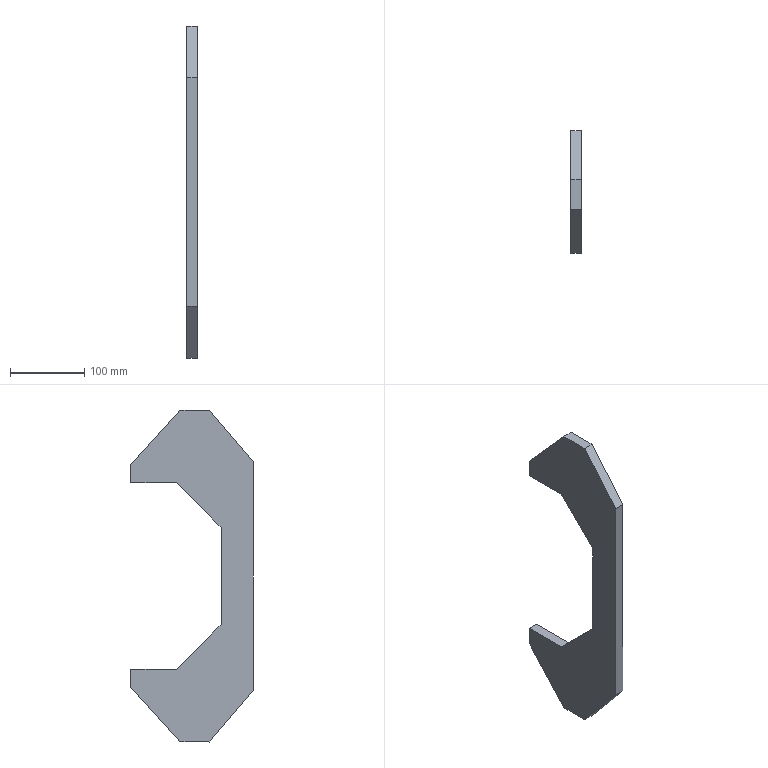Part | NX | features REPLACE_FACE 4, DATUM_CSYS 3, EXTRUDE 2, LINKED_FACE 2, SKETCH 2, BREP 1 | 1 solid | 16 faces | box 14 x 165.316 x 448 mm | volume 531264 mm3 | plane 16
STEP:
#1=CARTESIAN_POINT('',(116.,-146.,154.));
#2=VERTEX_POINT('',#1);
#3=CARTESIAN_POINT('',(116.,-146.,-154.));
#4=VERTEX_POINT('',#3);
#5=CARTESIAN_POINT('',(116.,-146.,154.));
#6=DIRECTION('',(0.,0.,-1.));
#7=VECTOR('',#6,1000.);
#8=LINE('',#5,#7);
#9=EDGE_CURVE('',#2,#4,#8,.T.);
#10=ORIENTED_EDGE('',*,*,#9,.F.);
#11=CARTESIAN_POINT('',(102.,-146.,154.));
#12=VERTEX_POINT('',#11);
#13=CARTESIAN_POINT('',(102.,-146.,154.));
#14=DIRECTION('',(1.,0.,0.));
#15=VECTOR('',#14,1000.);
#16=LINE('',#13,#15);
#17=EDGE_CURVE('',#12,#2,#16,.T.);
#18=ORIENTED_EDGE('',*,*,#17,.F.);
#19=CARTESIAN_POINT('',(102.,-146.,-154.));
#20=VERTEX_POINT('',#19);
#21=CARTESIAN_POINT('',(102.,-146.,154.));
#22=DIRECTION('',(0.,0.,-1.));
#23=VECTOR('',#22,1000.);
#24=LINE('',#21,#23);
#25=EDGE_CURVE('',#12,#20,#24,.T.);
#26=ORIENTED_EDGE('',*,*,#25,.T.);
#27=CARTESIAN_POINT('',(102.,-146.,-154.));
#28=DIRECTION('',(1.,0.,0.));
#29=VECTOR('',#28,1000.);
#30=LINE('',#27,#29);
#31=EDGE_CURVE('',#20,#4,#30,.T.);
#32=ORIENTED_EDGE('',*,*,#31,.T.);
#33=EDGE_LOOP('',(#10,#18,#26,#32));
#34=FACE_BOUND('',#33,.T.);
#35=CARTESIAN_POINT('',(102.,-146.,154.));
#36=DIRECTION('',(0.,-1.,0.));
#37=DIRECTION('',(0.,0.,-1.));
#38=AXIS2_PLACEMENT_3D('',#35,#36,#37);
#39=PLANE('',#38);
#40=ADVANCED_FACE('',(#34),#39,.T.);
#41=CARTESIAN_POINT('',(116.,-87.,-224.));
#42=VERTEX_POINT('',#41);
#43=CARTESIAN_POINT('',(116.,-146.,-154.));
#44=DIRECTION('',(0.,0.6445,-0.7646));
#45=VECTOR('',#44,1000.);
#46=LINE('',#43,#45);
#47=EDGE_CURVE('',#4,#42,#46,.T.);
#48=ORIENTED_EDGE('',*,*,#47,.F.);
#49=ORIENTED_EDGE('',*,*,#31,.F.);
#50=CARTESIAN_POINT('',(102.,-87.,-224.));
#51=VERTEX_POINT('',#50);
#52=CARTESIAN_POINT('',(102.,-146.,-154.));
#53=DIRECTION('',(0.,0.6445,-0.7646));
#54=VECTOR('',#53,1000.);
#55=LINE('',#52,#54);
#56=EDGE_CURVE('',#20,#51,#55,.T.);
#57=ORIENTED_EDGE('',*,*,#56,.T.);
#58=CARTESIAN_POINT('',(102.,-87.,-224.));
#59=DIRECTION('',(1.,0.,0.));
#60=VECTOR('',#59,1000.);
#61=LINE('',#58,#60);
#62=EDGE_CURVE('',#51,#42,#61,.T.);
#63=ORIENTED_EDGE('',*,*,#62,.T.);
#64=EDGE_LOOP('',(#48,#49,#57,#63));
#65=FACE_BOUND('',#64,.T.);
#66=CARTESIAN_POINT('',(102.,-146.,-154.));
#67=DIRECTION('',(0.,-0.7646,-0.6445));
#68=DIRECTION('',(0.,0.6445,-0.7646));
#69=AXIS2_PLACEMENT_3D('',#66,#67,#68);
#70=PLANE('',#69);
#71=ADVANCED_FACE('',(#65),#70,.T.);
#72=CARTESIAN_POINT('',(116.,-47.,-224.));
#73=VERTEX_POINT('',#72);
#74=CARTESIAN_POINT('',(116.,-87.,-224.));
#75=DIRECTION('',(0.,1.,0.));
#76=VECTOR('',#75,1000.);
#77=LINE('',#74,#76);
#78=EDGE_CURVE('',#42,#73,#77,.T.);
#79=ORIENTED_EDGE('',*,*,#78,.F.);
#80=ORIENTED_EDGE('',*,*,#62,.F.);
#81=CARTESIAN_POINT('',(102.,-47.,-224.));
#82=VERTEX_POINT('',#81);
#83=CARTESIAN_POINT('',(102.,-87.,-224.));
#84=DIRECTION('',(0.,1.,0.));
#85=VECTOR('',#84,1000.);
#86=LINE('',#83,#85);
#87=EDGE_CURVE('',#51,#82,#86,.T.);
#88=ORIENTED_EDGE('',*,*,#87,.T.);
#89=CARTESIAN_POINT('',(102.,-47.,-224.));
#90=DIRECTION('',(1.,0.,0.));
#91=VECTOR('',#90,1000.);
#92=LINE('',#89,#91);
#93=EDGE_CURVE('',#82,#73,#92,.T.);
#94=ORIENTED_EDGE('',*,*,#93,.T.);
#95=EDGE_LOOP('',(#79,#80,#88,#94));
#96=FACE_BOUND('',#95,.T.);
#97=CARTESIAN_POINT('',(102.,-87.,-224.));
#98=DIRECTION('',(0.,0.,-1.));
#99=DIRECTION('',(-1.,0.,0.));
#100=AXIS2_PLACEMENT_3D('',#97,#98,#99);
#101=PLANE('',#100);
#102=ADVANCED_FACE('',(#96),#101,.T.);
#103=CARTESIAN_POINT('',(116.,19.316,-150.316));
#104=VERTEX_POINT('',#103);
#105=CARTESIAN_POINT('',(116.,-47.,-224.));
#106=DIRECTION('',(0.,0.669,0.7433));
#107=VECTOR('',#106,1000.);
#108=LINE('',#105,#107);
#109=EDGE_CURVE('',#73,#104,#108,.T.);
#110=ORIENTED_EDGE('',*,*,#109,.F.);
#111=ORIENTED_EDGE('',*,*,#93,.F.);
#112=CARTESIAN_POINT('',(102.,19.316,-150.316));
#113=VERTEX_POINT('',#112);
#114=CARTESIAN_POINT('',(102.,-47.,-224.));
#115=DIRECTION('',(0.,0.669,0.7433));
#116=VECTOR('',#115,1000.);
#117=LINE('',#114,#116);
#118=EDGE_CURVE('',#82,#113,#117,.T.);
#119=ORIENTED_EDGE('',*,*,#118,.T.);
#120=CARTESIAN_POINT('',(102.,19.316,-150.316));
#121=DIRECTION('',(1.,0.,0.));
#122=VECTOR('',#121,1000.);
#123=LINE('',#120,#122);
#124=EDGE_CURVE('',#104,#113,#123,.F.);
#125=ORIENTED_EDGE('',*,*,#124,.F.);
#126=EDGE_LOOP('',(#110,#111,#119,#125));
#127=FACE_BOUND('',#126,.T.);
#128=CARTESIAN_POINT('',(102.,-47.,-224.));
#129=DIRECTION('',(0.,0.7433,-0.669));
#130=DIRECTION('',(0.,0.669,0.7433));
#131=AXIS2_PLACEMENT_3D('',#128,#129,#130);
#132=PLANE('',#131);
#133=ADVANCED_FACE('',(#127),#132,.T.);
#134=CARTESIAN_POINT('',(116.,19.316,-126.));
#135=VERTEX_POINT('',#134);
#136=CARTESIAN_POINT('',(116.,-42.5,-126.));
#137=VERTEX_POINT('',#136);
#138=CARTESIAN_POINT('',(116.,16.,-126.));
#139=DIRECTION('',(0.,-1.,0.));
#140=VECTOR('',#139,1000.);
#141=LINE('',#138,#140);
#142=EDGE_CURVE('',#135,#137,#141,.T.);
#143=ORIENTED_EDGE('',*,*,#142,.F.);
#144=CARTESIAN_POINT('',(102.,19.316,-126.));
#145=VERTEX_POINT('',#144);
#146=CARTESIAN_POINT('',(116.,19.316,-126.));
#147=DIRECTION('',(-1.,0.,0.));
#148=VECTOR('',#147,1000.);
#149=LINE('',#146,#148);
#150=EDGE_CURVE('',#135,#145,#149,.T.);
#151=ORIENTED_EDGE('',*,*,#150,.T.);
#152=CARTESIAN_POINT('',(102.,-42.5,-126.));
#153=VERTEX_POINT('',#152);
#154=CARTESIAN_POINT('',(102.,16.,-126.));
#155=DIRECTION('',(0.,-1.,0.));
#156=VECTOR('',#155,1000.);
#157=LINE('',#154,#156);
#158=EDGE_CURVE('',#145,#153,#157,.T.);
#159=ORIENTED_EDGE('',*,*,#158,.T.);
#160=CARTESIAN_POINT('',(102.,-42.5,-126.));
#161=DIRECTION('',(1.,0.,0.));
#162=VECTOR('',#161,1000.);
#163=LINE('',#160,#162);
#164=EDGE_CURVE('',#153,#137,#163,.T.);
#165=ORIENTED_EDGE('',*,*,#164,.T.);
#166=EDGE_LOOP('',(#143,#151,#159,#165));
#167=FACE_BOUND('',#166,.T.);
#168=CARTESIAN_POINT('',(102.,16.,-126.));
#169=DIRECTION('',(0.,0.,1.));
#170=DIRECTION('',(1.,0.,0.));
#171=AXIS2_PLACEMENT_3D('',#168,#169,#170);
#172=PLANE('',#171);
#173=ADVANCED_FACE('',(#167),#172,.T.);
#174=CARTESIAN_POINT('',(116.,-102.5,-66.));
#175=VERTEX_POINT('',#174);
#176=CARTESIAN_POINT('',(116.,-42.5,-126.));
#177=DIRECTION('',(0.,-0.7071,0.7071));
#178=VECTOR('',#177,1000.);
#179=LINE('',#176,#178);
#180=EDGE_CURVE('',#137,#175,#179,.T.);
#181=ORIENTED_EDGE('',*,*,#180,.F.);
#182=ORIENTED_EDGE('',*,*,#164,.F.);
#183=CARTESIAN_POINT('',(102.,-102.5,-66.));
#184=VERTEX_POINT('',#183);
#185=CARTESIAN_POINT('',(102.,-42.5,-126.));
#186=DIRECTION('',(0.,-0.7071,0.7071));
#187=VECTOR('',#186,1000.);
#188=LINE('',#185,#187);
#189=EDGE_CURVE('',#153,#184,#188,.T.);
#190=ORIENTED_EDGE('',*,*,#189,.T.);
#191=CARTESIAN_POINT('',(102.,-102.5,-66.));
#192=DIRECTION('',(1.,0.,0.));
#193=VECTOR('',#192,1000.);
#194=LINE('',#191,#193);
#195=EDGE_CURVE('',#184,#175,#194,.T.);
#196=ORIENTED_EDGE('',*,*,#195,.T.);
#197=EDGE_LOOP('',(#181,#182,#190,#196));
#198=FACE_BOUND('',#197,.T.);
#199=CARTESIAN_POINT('',(102.,-42.5,-126.));
#200=DIRECTION('',(0.,0.7071,0.7071));
#201=DIRECTION('',(0.,-0.7071,0.7071));
#202=AXIS2_PLACEMENT_3D('',#199,#200,#201);
#203=PLANE('',#202);
#204=ADVANCED_FACE('',(#198),#203,.T.);
#205=CARTESIAN_POINT('',(116.,-102.5,66.));
#206=VERTEX_POINT('',#205);
#207=CARTESIAN_POINT('',(116.,-102.5,-66.));
#208=DIRECTION('',(0.,0.,1.));
#209=VECTOR('',#208,1000.);
#210=LINE('',#207,#209);
#211=EDGE_CURVE('',#175,#206,#210,.T.);
#212=ORIENTED_EDGE('',*,*,#211,.F.);
#213=ORIENTED_EDGE('',*,*,#195,.F.);
#214=CARTESIAN_POINT('',(102.,-102.5,66.));
#215=VERTEX_POINT('',#214);
#216=CARTESIAN_POINT('',(102.,-102.5,-66.));
#217=DIRECTION('',(0.,0.,1.));
#218=VECTOR('',#217,1000.);
#219=LINE('',#216,#218);
#220=EDGE_CURVE('',#184,#215,#219,.T.);
#221=ORIENTED_EDGE('',*,*,#220,.T.);
#222=CARTESIAN_POINT('',(102.,-102.5,66.));
#223=DIRECTION('',(1.,0.,0.));
#224=VECTOR('',#223,1000.);
#225=LINE('',#222,#224);
#226=EDGE_CURVE('',#215,#206,#225,.T.);
#227=ORIENTED_EDGE('',*,*,#226,.T.);
#228=EDGE_LOOP('',(#212,#213,#221,#227));
#229=FACE_BOUND('',#228,.T.);
#230=CARTESIAN_POINT('',(102.,-102.5,-66.));
#231=DIRECTION('',(0.,1.,0.));
#232=DIRECTION('',(0.,0.,1.));
#233=AXIS2_PLACEMENT_3D('',#230,#231,#232);
#234=PLANE('',#233);
#235=ADVANCED_FACE('',(#229),#234,.T.);
#236=CARTESIAN_POINT('',(116.,-42.5,126.));
#237=VERTEX_POINT('',#236);
#238=CARTESIAN_POINT('',(116.,-102.5,66.));
#239=DIRECTION('',(0.,0.7071,0.7071));
#240=VECTOR('',#239,1000.);
#241=LINE('',#238,#240);
#242=EDGE_CURVE('',#206,#237,#241,.T.);
#243=ORIENTED_EDGE('',*,*,#242,.F.);
#244=ORIENTED_EDGE('',*,*,#226,.F.);
#245=CARTESIAN_POINT('',(102.,-42.5,126.));
#246=VERTEX_POINT('',#245);
#247=CARTESIAN_POINT('',(102.,-102.5,66.));
#248=DIRECTION('',(0.,0.7071,0.7071));
#249=VECTOR('',#248,1000.);
#250=LINE('',#247,#249);
#251=EDGE_CURVE('',#215,#246,#250,.T.);
#252=ORIENTED_EDGE('',*,*,#251,.T.);
#253=CARTESIAN_POINT('',(102.,-42.5,126.));
#254=DIRECTION('',(1.,0.,0.));
#255=VECTOR('',#254,1000.);
#256=LINE('',#253,#255);
#257=EDGE_CURVE('',#246,#237,#256,.T.);
#258=ORIENTED_EDGE('',*,*,#257,.T.);
#259=EDGE_LOOP('',(#243,#244,#252,#258));
#260=FACE_BOUND('',#259,.T.);
#261=CARTESIAN_POINT('',(102.,-102.5,66.));
#262=DIRECTION('',(0.,0.7071,-0.7071));
#263=DIRECTION('',(0.,0.7071,0.7071));
#264=AXIS2_PLACEMENT_3D('',#261,#262,#263);
#265=PLANE('',#264);
#266=ADVANCED_FACE('',(#260),#265,.T.);
#267=CARTESIAN_POINT('',(116.,19.316,126.));
#268=VERTEX_POINT('',#267);
#269=CARTESIAN_POINT('',(116.,-42.5,126.));
#270=DIRECTION('',(0.,1.,0.));
#271=VECTOR('',#270,1000.);
#272=LINE('',#269,#271);
#273=EDGE_CURVE('',#237,#268,#272,.T.);
#274=ORIENTED_EDGE('',*,*,#273,.F.);
#275=ORIENTED_EDGE('',*,*,#257,.F.);
#276=CARTESIAN_POINT('',(102.,19.316,126.));
#277=VERTEX_POINT('',#276);
#278=CARTESIAN_POINT('',(102.,-42.5,126.));
#279=DIRECTION('',(0.,1.,0.));
#280=VECTOR('',#279,1000.);
#281=LINE('',#278,#280);
#282=EDGE_CURVE('',#246,#277,#281,.T.);
#283=ORIENTED_EDGE('',*,*,#282,.T.);
#284=CARTESIAN_POINT('',(102.,19.316,126.));
#285=DIRECTION('',(1.,0.,0.));
#286=VECTOR('',#285,1000.);
#287=LINE('',#284,#286);
#288=EDGE_CURVE('',#277,#268,#287,.T.);
#289=ORIENTED_EDGE('',*,*,#288,.T.);
#290=EDGE_LOOP('',(#274,#275,#283,#289));
#291=FACE_BOUND('',#290,.T.);
#292=CARTESIAN_POINT('',(102.,-42.5,126.));
#293=DIRECTION('',(0.,0.,-1.));
#294=DIRECTION('',(-1.,0.,0.));
#295=AXIS2_PLACEMENT_3D('',#292,#293,#294);
#296=PLANE('',#295);
#297=ADVANCED_FACE('',(#291),#296,.T.);
#298=CARTESIAN_POINT('',(116.,19.316,150.316));
#299=VERTEX_POINT('',#298);
#300=CARTESIAN_POINT('',(116.,-47.,224.));
#301=VERTEX_POINT('',#300);
#302=CARTESIAN_POINT('',(116.,16.,154.));
#303=DIRECTION('',(0.,-0.669,0.7433));
#304=VECTOR('',#303,1000.);
#305=LINE('',#302,#304);
#306=EDGE_CURVE('',#299,#301,#305,.T.);
#307=ORIENTED_EDGE('',*,*,#306,.F.);
#308=CARTESIAN_POINT('',(102.,19.316,150.316));
#309=VERTEX_POINT('',#308);
#310=CARTESIAN_POINT('',(102.,19.316,150.316));
#311=DIRECTION('',(1.,0.,0.));
#312=VECTOR('',#311,1000.);
#313=LINE('',#310,#312);
#314=EDGE_CURVE('',#309,#299,#313,.T.);
#315=ORIENTED_EDGE('',*,*,#314,.F.);
#316=CARTESIAN_POINT('',(102.,-47.,224.));
#317=VERTEX_POINT('',#316);
#318=CARTESIAN_POINT('',(102.,16.,154.));
#319=DIRECTION('',(0.,-0.669,0.7433));
#320=VECTOR('',#319,1000.);
#321=LINE('',#318,#320);
#322=EDGE_CURVE('',#309,#317,#321,.T.);
#323=ORIENTED_EDGE('',*,*,#322,.T.);
#324=CARTESIAN_POINT('',(102.,-47.,224.));
#325=DIRECTION('',(1.,0.,0.));
#326=VECTOR('',#325,1000.);
#327=LINE('',#324,#326);
#328=EDGE_CURVE('',#317,#301,#327,.T.);
#329=ORIENTED_EDGE('',*,*,#328,.T.);
#330=EDGE_LOOP('',(#307,#315,#323,#329));
#331=FACE_BOUND('',#330,.T.);
#332=CARTESIAN_POINT('',(102.,16.,154.));
#333=DIRECTION('',(0.,0.7433,0.669));
#334=DIRECTION('',(0.,-0.669,0.7433));
#335=AXIS2_PLACEMENT_3D('',#332,#333,#334);
#336=PLANE('',#335);
#337=ADVANCED_FACE('',(#331),#336,.T.);
#338=CARTESIAN_POINT('',(116.,-87.,224.));
#339=VERTEX_POINT('',#338);
#340=CARTESIAN_POINT('',(116.,-47.,224.));
#341=DIRECTION('',(0.,-1.,0.));
#342=VECTOR('',#341,1000.);
#343=LINE('',#340,#342);
#344=EDGE_CURVE('',#301,#339,#343,.T.);
#345=ORIENTED_EDGE('',*,*,#344,.F.);
#346=ORIENTED_EDGE('',*,*,#328,.F.);
#347=CARTESIAN_POINT('',(102.,-87.,224.));
#348=VERTEX_POINT('',#347);
#349=CARTESIAN_POINT('',(102.,-47.,224.));
#350=DIRECTION('',(0.,-1.,0.));
#351=VECTOR('',#350,1000.);
#352=LINE('',#349,#351);
#353=EDGE_CURVE('',#317,#348,#352,.T.);
#354=ORIENTED_EDGE('',*,*,#353,.T.);
#355=CARTESIAN_POINT('',(102.,-87.,224.));
#356=DIRECTION('',(1.,0.,0.));
#357=VECTOR('',#356,1000.);
#358=LINE('',#355,#357);
#359=EDGE_CURVE('',#348,#339,#358,.T.);
#360=ORIENTED_EDGE('',*,*,#359,.T.);
#361=EDGE_LOOP('',(#345,#346,#354,#360));
#362=FACE_BOUND('',#361,.T.);
#363=CARTESIAN_POINT('',(102.,-47.,224.));
#364=DIRECTION('',(0.,0.,1.));
#365=DIRECTION('',(1.,0.,0.));
#366=AXIS2_PLACEMENT_3D('',#363,#364,#365);
#367=PLANE('',#366);
#368=ADVANCED_FACE('',(#362),#367,.T.);
#369=CARTESIAN_POINT('',(116.,-87.,224.));
#370=DIRECTION('',(0.,-0.6445,-0.7646));
#371=VECTOR('',#370,1000.);
#372=LINE('',#369,#371);
#373=EDGE_CURVE('',#339,#2,#372,.T.);
#374=ORIENTED_EDGE('',*,*,#373,.F.);
#375=ORIENTED_EDGE('',*,*,#359,.F.);
#376=CARTESIAN_POINT('',(102.,-87.,224.));
#377=DIRECTION('',(0.,-0.6445,-0.7646));
#378=VECTOR('',#377,1000.);
#379=LINE('',#376,#378);
#380=EDGE_CURVE('',#348,#12,#379,.T.);
#381=ORIENTED_EDGE('',*,*,#380,.T.);
#382=ORIENTED_EDGE('',*,*,#17,.T.);
#383=EDGE_LOOP('',(#374,#375,#381,#382));
#384=FACE_BOUND('',#383,.T.);
#385=CARTESIAN_POINT('',(102.,-87.,224.));
#386=DIRECTION('',(0.,-0.7646,0.6445));
#387=DIRECTION('',(0.,-0.6445,-0.7646));
#388=AXIS2_PLACEMENT_3D('',#385,#386,#387);
#389=PLANE('',#388);
#390=ADVANCED_FACE('',(#384),#389,.T.);
#391=ORIENTED_EDGE('',*,*,#25,.F.);
#392=ORIENTED_EDGE('',*,*,#380,.F.);
#393=ORIENTED_EDGE('',*,*,#353,.F.);
#394=ORIENTED_EDGE('',*,*,#322,.F.);
#395=CARTESIAN_POINT('',(102.,19.316,0.));
#396=DIRECTION('',(0.,0.,1.));
#397=VECTOR('',#396,1000.);
#398=LINE('',#395,#397);
#399=EDGE_CURVE('',#277,#309,#398,.T.);
#400=ORIENTED_EDGE('',*,*,#399,.F.);
#401=ORIENTED_EDGE('',*,*,#282,.F.);
#402=ORIENTED_EDGE('',*,*,#251,.F.);
#403=ORIENTED_EDGE('',*,*,#220,.F.);
#404=ORIENTED_EDGE('',*,*,#189,.F.);
#405=ORIENTED_EDGE('',*,*,#158,.F.);
#406=CARTESIAN_POINT('',(102.,19.316,0.));
#407=DIRECTION('',(0.,0.,1.));
#408=VECTOR('',#407,1000.);
#409=LINE('',#406,#408);
#410=EDGE_CURVE('',#113,#145,#409,.T.);
#411=ORIENTED_EDGE('',*,*,#410,.F.);
#412=ORIENTED_EDGE('',*,*,#118,.F.);
#413=ORIENTED_EDGE('',*,*,#87,.F.);
#414=ORIENTED_EDGE('',*,*,#56,.F.);
#415=EDGE_LOOP('',(#391,#392,#393,#394,#400,#401,#402,#403,#404,#405,#411,#412,#413,#414));
#416=FACE_BOUND('',#415,.T.);
#417=CARTESIAN_POINT('',(102.,0.,0.));
#418=DIRECTION('',(1.,0.,0.));
#419=DIRECTION('',(0.,0.,-1.));
#420=AXIS2_PLACEMENT_3D('',#417,#418,#419);
#421=PLANE('',#420);
#422=ADVANCED_FACE('',(#416),#421,.F.);
#423=ORIENTED_EDGE('',*,*,#9,.T.);
#424=ORIENTED_EDGE('',*,*,#47,.T.);
#425=ORIENTED_EDGE('',*,*,#78,.T.);
#426=ORIENTED_EDGE('',*,*,#109,.T.);
#427=CARTESIAN_POINT('',(116.,19.316,-154.));
#428=DIRECTION('',(0.,0.,1.));
#429=VECTOR('',#428,1000.);
#430=LINE('',#427,#429);
#431=EDGE_CURVE('',#104,#135,#430,.T.);
#432=ORIENTED_EDGE('',*,*,#431,.T.);
#433=ORIENTED_EDGE('',*,*,#142,.T.);
#434=ORIENTED_EDGE('',*,*,#180,.T.);
#435=ORIENTED_EDGE('',*,*,#211,.T.);
#436=ORIENTED_EDGE('',*,*,#242,.T.);
#437=ORIENTED_EDGE('',*,*,#273,.T.);
#438=CARTESIAN_POINT('',(116.,19.316,154.));
#439=DIRECTION('',(0.,0.,-1.));
#440=VECTOR('',#439,1000.);
#441=LINE('',#438,#440);
#442=EDGE_CURVE('',#299,#268,#441,.T.);
#443=ORIENTED_EDGE('',*,*,#442,.F.);
#444=ORIENTED_EDGE('',*,*,#306,.T.);
#445=ORIENTED_EDGE('',*,*,#344,.T.);
#446=ORIENTED_EDGE('',*,*,#373,.T.);
#447=EDGE_LOOP('',(#423,#424,#425,#426,#432,#433,#434,#435,#436,#437,#443,#444,#445,#446));
#448=FACE_BOUND('',#447,.T.);
#449=CARTESIAN_POINT('',(116.,0.,0.));
#450=DIRECTION('',(1.,0.,0.));
#451=DIRECTION('',(0.,0.,-1.));
#452=AXIS2_PLACEMENT_3D('',#449,#450,#451);
#453=PLANE('',#452);
#454=ADVANCED_FACE('',(#448),#453,.T.);
#455=ORIENTED_EDGE('',*,*,#150,.F.);
#456=ORIENTED_EDGE('',*,*,#431,.F.);
#457=ORIENTED_EDGE('',*,*,#124,.T.);
#458=ORIENTED_EDGE('',*,*,#410,.T.);
#459=EDGE_LOOP('',(#455,#456,#457,#458));
#460=FACE_BOUND('',#459,.T.);
#461=CARTESIAN_POINT('',(116.,19.316,-154.));
#462=DIRECTION('',(0.,1.,0.));
#463=DIRECTION('',(0.,0.,1.));
#464=AXIS2_PLACEMENT_3D('',#461,#462,#463);
#465=PLANE('',#464);
#466=ADVANCED_FACE('',(#460),#465,.T.);
#467=ORIENTED_EDGE('',*,*,#288,.F.);
#468=ORIENTED_EDGE('',*,*,#399,.T.);
#469=ORIENTED_EDGE('',*,*,#314,.T.);
#470=ORIENTED_EDGE('',*,*,#442,.T.);
#471=EDGE_LOOP('',(#467,#468,#469,#470));
#472=FACE_BOUND('',#471,.T.);
#473=CARTESIAN_POINT('',(102.,19.316,154.));
#474=DIRECTION('',(0.,1.,0.));
#475=DIRECTION('',(-1.,0.,0.));
#476=AXIS2_PLACEMENT_3D('',#473,#474,#475);
#477=PLANE('',#476);
#478=ADVANCED_FACE('',(#472),#477,.T.);
#479=CLOSED_SHELL('',(#40,#71,#102,#133,#173,#204,#235,#266,#297,#337,#368,#390,#422,#454,#466,#478));
#480=MANIFOLD_SOLID_BREP('',#479);
#481=(LENGTH_UNIT()NAMED_UNIT(*)SI_UNIT(.MILLI.,.METRE.));
#482=UNCERTAINTY_MEASURE_WITH_UNIT(LENGTH_MEASURE(0.00001),#481,'','');
#483=(NAMED_UNIT(*)PLANE_ANGLE_UNIT()SI_UNIT($,.RADIAN.));
#484=(NAMED_UNIT(*)SI_UNIT($,.STERADIAN.)SOLID_ANGLE_UNIT());
#485=(GEOMETRIC_REPRESENTATION_CONTEXT(3)GLOBAL_UNCERTAINTY_ASSIGNED_CONTEXT((#482))GLOBAL_UNIT_ASSIGNED_CONTEXT((#481,#483,#484))REPRESENTATION_CONTEXT('',''));
#486=ADVANCED_BREP_SHAPE_REPRESENTATION('',(#480),#485);